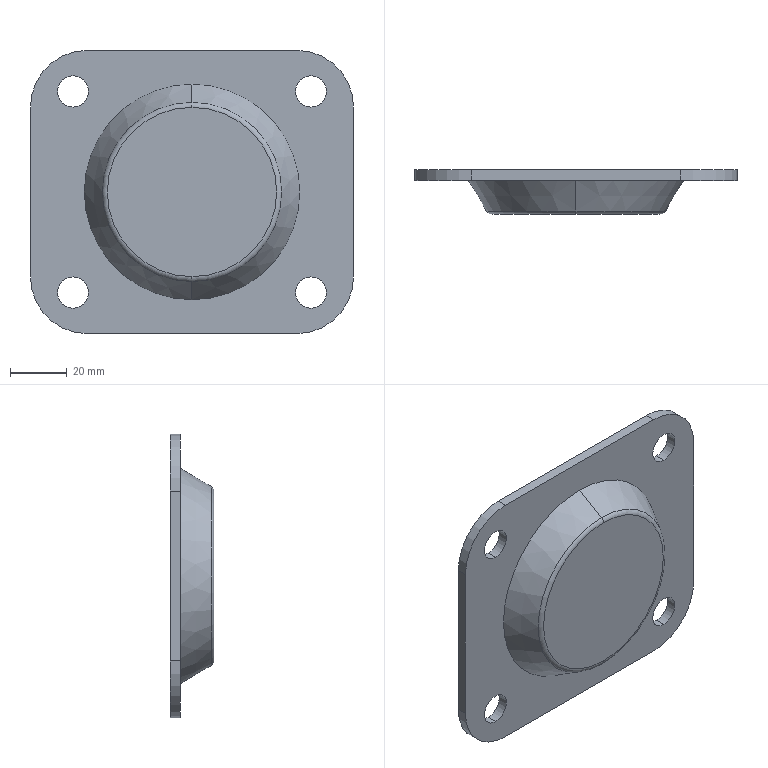Part | SolidWorks | features RefAxis 6, 3DProfileFeature 2, ICE 2, Extrusion 1, Revolution 1 | 1 solid | 26 faces | box 114 x 15.475 x 100 mm | volume 79826 mm3 | cylinder 14 | plane 8 | torus 2 | cone 2 | commonest cylinder face diameters 11 x8 40 x4 63.333 x2
STEP:
#1=CARTESIAN_POINT('',(-42.,-3.6,30.));
#2=VERTEX_POINT('',#1);
#3=CARTESIAN_POINT('',(-42.,-3.6,41.));
#4=VERTEX_POINT('',#3);
#5=CARTESIAN_POINT('',(-42.,-3.6,35.5));
#6=DIRECTION('',(0.,1.,0.));
#7=DIRECTION('',(0.,0.,1.));
#8=AXIS2_PLACEMENT_3D('',#5,#6,#7);
#9=CIRCLE('',#8,5.5);
#10=EDGE_CURVE('',#2,#4,#9,.T.);
#11=ORIENTED_EDGE('',*,*,#10,.F.);
#12=CARTESIAN_POINT('',(-42.,0.,30.));
#13=VERTEX_POINT('',#12);
#14=CARTESIAN_POINT('',(-42.,-15.475,30.));
#15=DIRECTION('',(0.,1.,0.));
#16=VECTOR('',#15,1000.);
#17=LINE('',#14,#16);
#18=EDGE_CURVE('',#2,#13,#17,.T.);
#19=ORIENTED_EDGE('',*,*,#18,.T.);
#20=CARTESIAN_POINT('',(-42.,0.,41.));
#21=VERTEX_POINT('',#20);
#22=CARTESIAN_POINT('',(-42.,0.,35.5));
#23=DIRECTION('',(0.,1.,0.));
#24=DIRECTION('',(0.,0.,-1.));
#25=AXIS2_PLACEMENT_3D('',#22,#23,#24);
#26=CIRCLE('',#25,5.5);
#27=EDGE_CURVE('',#13,#21,#26,.T.);
#28=ORIENTED_EDGE('',*,*,#27,.T.);
#29=CARTESIAN_POINT('',(-42.,-15.475,41.));
#30=DIRECTION('',(0.,1.,0.));
#31=VECTOR('',#30,1000.);
#32=LINE('',#29,#31);
#33=EDGE_CURVE('',#4,#21,#32,.T.);
#34=ORIENTED_EDGE('',*,*,#33,.F.);
#35=EDGE_LOOP('',(#11,#19,#28,#34));
#36=FACE_OUTER_BOUND('',#35,.T.);
#37=CARTESIAN_POINT('',(-42.,-15.475,35.5));
#38=DIRECTION('',(0.,1.,0.));
#39=DIRECTION('',(0.,0.,1.));
#40=AXIS2_PLACEMENT_3D('',#37,#38,#39);
#41=CYLINDRICAL_SURFACE('',#40,5.5);
#42=ADVANCED_FACE('',(#36),#41,.F.);
#43=CARTESIAN_POINT('',(42.,-3.6,30.));
#44=VERTEX_POINT('',#43);
#45=CARTESIAN_POINT('',(42.,-3.6,41.));
#46=VERTEX_POINT('',#45);
#47=CARTESIAN_POINT('',(42.,-3.6,35.5));
#48=DIRECTION('',(0.,1.,0.));
#49=DIRECTION('',(0.,0.,1.));
#50=AXIS2_PLACEMENT_3D('',#47,#48,#49);
#51=CIRCLE('',#50,5.5);
#52=EDGE_CURVE('',#44,#46,#51,.T.);
#53=ORIENTED_EDGE('',*,*,#52,.F.);
#54=CARTESIAN_POINT('',(42.,0.,30.));
#55=VERTEX_POINT('',#54);
#56=CARTESIAN_POINT('',(42.,-15.475,30.));
#57=DIRECTION('',(0.,1.,0.));
#58=VECTOR('',#57,1000.);
#59=LINE('',#56,#58);
#60=EDGE_CURVE('',#44,#55,#59,.T.);
#61=ORIENTED_EDGE('',*,*,#60,.T.);
#62=CARTESIAN_POINT('',(42.,0.,41.));
#63=VERTEX_POINT('',#62);
#64=CARTESIAN_POINT('',(42.,0.,35.5));
#65=DIRECTION('',(0.,1.,0.));
#66=DIRECTION('',(0.,0.,-1.));
#67=AXIS2_PLACEMENT_3D('',#64,#65,#66);
#68=CIRCLE('',#67,5.5);
#69=EDGE_CURVE('',#55,#63,#68,.T.);
#70=ORIENTED_EDGE('',*,*,#69,.T.);
#71=CARTESIAN_POINT('',(42.,-15.475,41.));
#72=DIRECTION('',(0.,1.,0.));
#73=VECTOR('',#72,1000.);
#74=LINE('',#71,#73);
#75=EDGE_CURVE('',#46,#63,#74,.T.);
#76=ORIENTED_EDGE('',*,*,#75,.F.);
#77=EDGE_LOOP('',(#53,#61,#70,#76));
#78=FACE_OUTER_BOUND('',#77,.T.);
#79=CARTESIAN_POINT('',(42.,-15.475,35.5));
#80=DIRECTION('',(0.,1.,0.));
#81=DIRECTION('',(0.,0.,1.));
#82=AXIS2_PLACEMENT_3D('',#79,#80,#81);
#83=CYLINDRICAL_SURFACE('',#82,5.5);
#84=ADVANCED_FACE('',(#78),#83,.F.);
#85=CARTESIAN_POINT('',(42.,-3.6,-41.));
#86=VERTEX_POINT('',#85);
#87=CARTESIAN_POINT('',(42.,-3.6,-30.));
#88=VERTEX_POINT('',#87);
#89=CARTESIAN_POINT('',(42.,-3.6,-35.5));
#90=DIRECTION('',(0.,1.,0.));
#91=DIRECTION('',(0.,0.,1.));
#92=AXIS2_PLACEMENT_3D('',#89,#90,#91);
#93=CIRCLE('',#92,5.5);
#94=EDGE_CURVE('',#86,#88,#93,.T.);
#95=ORIENTED_EDGE('',*,*,#94,.F.);
#96=CARTESIAN_POINT('',(42.,0.,-41.));
#97=VERTEX_POINT('',#96);
#98=CARTESIAN_POINT('',(42.,-15.475,-41.));
#99=DIRECTION('',(0.,1.,0.));
#100=VECTOR('',#99,1000.);
#101=LINE('',#98,#100);
#102=EDGE_CURVE('',#86,#97,#101,.T.);
#103=ORIENTED_EDGE('',*,*,#102,.T.);
#104=CARTESIAN_POINT('',(42.,0.,-30.));
#105=VERTEX_POINT('',#104);
#106=CARTESIAN_POINT('',(42.,0.,-35.5));
#107=DIRECTION('',(0.,1.,0.));
#108=DIRECTION('',(0.,0.,1.));
#109=AXIS2_PLACEMENT_3D('',#106,#107,#108);
#110=CIRCLE('',#109,5.5);
#111=EDGE_CURVE('',#97,#105,#110,.T.);
#112=ORIENTED_EDGE('',*,*,#111,.T.);
#113=CARTESIAN_POINT('',(42.,-15.475,-30.));
#114=DIRECTION('',(0.,1.,0.));
#115=VECTOR('',#114,1000.);
#116=LINE('',#113,#115);
#117=EDGE_CURVE('',#88,#105,#116,.T.);
#118=ORIENTED_EDGE('',*,*,#117,.F.);
#119=EDGE_LOOP('',(#95,#103,#112,#118));
#120=FACE_OUTER_BOUND('',#119,.T.);
#121=CARTESIAN_POINT('',(42.,-15.475,-35.5));
#122=DIRECTION('',(0.,1.,0.));
#123=DIRECTION('',(0.,0.,1.));
#124=AXIS2_PLACEMENT_3D('',#121,#122,#123);
#125=CYLINDRICAL_SURFACE('',#124,5.5);
#126=ADVANCED_FACE('',(#120),#125,.F.);
#127=CARTESIAN_POINT('',(-42.,-3.6,-41.));
#128=VERTEX_POINT('',#127);
#129=CARTESIAN_POINT('',(-42.,-3.6,-30.));
#130=VERTEX_POINT('',#129);
#131=CARTESIAN_POINT('',(-42.,-3.6,-35.5));
#132=DIRECTION('',(0.,1.,0.));
#133=DIRECTION('',(0.,0.,1.));
#134=AXIS2_PLACEMENT_3D('',#131,#132,#133);
#135=CIRCLE('',#134,5.5);
#136=EDGE_CURVE('',#128,#130,#135,.T.);
#137=ORIENTED_EDGE('',*,*,#136,.F.);
#138=CARTESIAN_POINT('',(-42.,0.,-41.));
#139=VERTEX_POINT('',#138);
#140=CARTESIAN_POINT('',(-42.,-15.475,-41.));
#141=DIRECTION('',(0.,1.,0.));
#142=VECTOR('',#141,1000.);
#143=LINE('',#140,#142);
#144=EDGE_CURVE('',#128,#139,#143,.T.);
#145=ORIENTED_EDGE('',*,*,#144,.T.);
#146=CARTESIAN_POINT('',(-42.,0.,-30.));
#147=VERTEX_POINT('',#146);
#148=CARTESIAN_POINT('',(-42.,0.,-35.5));
#149=DIRECTION('',(0.,1.,0.));
#150=DIRECTION('',(0.,0.,1.));
#151=AXIS2_PLACEMENT_3D('',#148,#149,#150);
#152=CIRCLE('',#151,5.5);
#153=EDGE_CURVE('',#139,#147,#152,.T.);
#154=ORIENTED_EDGE('',*,*,#153,.T.);
#155=CARTESIAN_POINT('',(-42.,-15.475,-30.));
#156=DIRECTION('',(0.,1.,0.));
#157=VECTOR('',#156,1000.);
#158=LINE('',#155,#157);
#159=EDGE_CURVE('',#130,#147,#158,.T.);
#160=ORIENTED_EDGE('',*,*,#159,.F.);
#161=EDGE_LOOP('',(#137,#145,#154,#160));
#162=FACE_OUTER_BOUND('',#161,.T.);
#163=CARTESIAN_POINT('',(-42.,-15.475,-35.5));
#164=DIRECTION('',(0.,1.,0.));
#165=DIRECTION('',(0.,0.,1.));
#166=AXIS2_PLACEMENT_3D('',#163,#164,#165);
#167=CYLINDRICAL_SURFACE('',#166,5.5);
#168=ADVANCED_FACE('',(#162),#167,.F.);
#169=CARTESIAN_POINT('',(0.,-15.475,29.876));
#170=VERTEX_POINT('',#169);
#171=CARTESIAN_POINT('',(0.,-15.475,-29.876));
#172=VERTEX_POINT('',#171);
#173=CARTESIAN_POINT('',(0.,-15.475,0.));
#174=DIRECTION('',(0.,1.,0.));
#175=DIRECTION('',(0.,0.,1.));
#176=AXIS2_PLACEMENT_3D('',#173,#174,#175);
#177=CIRCLE('',#176,29.876);
#178=EDGE_CURVE('',#170,#172,#177,.T.);
#179=ORIENTED_EDGE('',*,*,#178,.T.);
#180=CARTESIAN_POINT('',(0.,-14.488,-31.6));
#181=VERTEX_POINT('',#180);
#182=CARTESIAN_POINT('',(0.,-13.475,-29.876));
#183=DIRECTION('',(1.,0.,0.));
#184=DIRECTION('',(0.,0.,-1.));
#185=AXIS2_PLACEMENT_3D('',#182,#183,#184);
#186=CIRCLE('',#185,2.);
#187=EDGE_CURVE('',#172,#181,#186,.T.);
#188=ORIENTED_EDGE('',*,*,#187,.T.);
#189=CARTESIAN_POINT('',(0.,-14.488,31.6));
#190=VERTEX_POINT('',#189);
#191=CARTESIAN_POINT('',(0.,-14.488,0.));
#192=DIRECTION('',(0.,1.,0.));
#193=DIRECTION('',(0.,0.,1.));
#194=AXIS2_PLACEMENT_3D('',#191,#192,#193);
#195=CIRCLE('',#194,31.6);
#196=EDGE_CURVE('',#190,#181,#195,.T.);
#197=ORIENTED_EDGE('',*,*,#196,.F.);
#198=CARTESIAN_POINT('',(0.,-13.475,29.876));
#199=DIRECTION('',(-1.,0.,0.));
#200=DIRECTION('',(0.,0.,1.));
#201=AXIS2_PLACEMENT_3D('',#198,#199,#200);
#202=CIRCLE('',#201,2.);
#203=EDGE_CURVE('',#170,#190,#202,.T.);
#204=ORIENTED_EDGE('',*,*,#203,.F.);
#205=EDGE_LOOP('',(#179,#188,#197,#204));
#206=FACE_OUTER_BOUND('',#205,.T.);
#207=CARTESIAN_POINT('',(0.,-13.475,0.));
#208=DIRECTION('',(0.,1.,0.));
#209=DIRECTION('',(0.,0.,1.));
#210=AXIS2_PLACEMENT_3D('',#207,#208,#209);
#211=TOROIDAL_SURFACE('',#210,29.876,2.);
#212=ADVANCED_FACE('',(#206),#211,.T.);
#213=ORIENTED_EDGE('',*,*,#196,.T.);
#214=CARTESIAN_POINT('',(0.,-3.6,-38.));
#215=VERTEX_POINT('',#214);
#216=CARTESIAN_POINT('',(0.,-14.488,-31.6));
#217=DIRECTION('',(0.,0.8621,-0.5067));
#218=VECTOR('',#217,1000.);
#219=LINE('',#216,#218);
#220=EDGE_CURVE('',#181,#215,#219,.T.);
#221=ORIENTED_EDGE('',*,*,#220,.T.);
#222=CARTESIAN_POINT('',(0.,-3.6,38.));
#223=VERTEX_POINT('',#222);
#224=CARTESIAN_POINT('',(0.,-3.6,0.));
#225=DIRECTION('',(0.,-1.,0.));
#226=DIRECTION('',(0.,0.,1.));
#227=AXIS2_PLACEMENT_3D('',#224,#225,#226);
#228=CIRCLE('',#227,38.);
#229=EDGE_CURVE('',#215,#223,#228,.T.);
#230=ORIENTED_EDGE('',*,*,#229,.T.);
#231=CARTESIAN_POINT('',(0.,-14.488,31.6));
#232=DIRECTION('',(0.,0.8621,0.5067));
#233=VECTOR('',#232,1000.);
#234=LINE('',#231,#233);
#235=EDGE_CURVE('',#190,#223,#234,.T.);
#236=ORIENTED_EDGE('',*,*,#235,.F.);
#237=EDGE_LOOP('',(#213,#221,#230,#236));
#238=FACE_OUTER_BOUND('',#237,.T.);
#239=CARTESIAN_POINT('',(0.,-14.488,0.));
#240=DIRECTION('',(0.,1.,0.));
#241=DIRECTION('',(0.,0.,1.));
#242=AXIS2_PLACEMENT_3D('',#239,#240,#241);
#243=CONICAL_SURFACE('',#242,31.6,0.5314);
#244=ADVANCED_FACE('',(#238),#243,.T.);
#245=CARTESIAN_POINT('',(0.,-1.,-31.667));
#246=VERTEX_POINT('',#245);
#247=CARTESIAN_POINT('',(0.,-1.,31.667));
#248=VERTEX_POINT('',#247);
#249=CARTESIAN_POINT('',(0.,-1.,0.));
#250=DIRECTION('',(0.,1.,0.));
#251=DIRECTION('',(0.,0.,1.));
#252=AXIS2_PLACEMENT_3D('',#249,#250,#251);
#253=CIRCLE('',#252,31.667);
#254=EDGE_CURVE('',#246,#248,#253,.T.);
#255=ORIENTED_EDGE('',*,*,#254,.F.);
#256=CARTESIAN_POINT('',(0.,0.,-31.667));
#257=VERTEX_POINT('',#256);
#258=CARTESIAN_POINT('',(0.,-1.,-31.667));
#259=DIRECTION('',(0.,1.,0.));
#260=VECTOR('',#259,1000.);
#261=LINE('',#258,#260);
#262=EDGE_CURVE('',#246,#257,#261,.T.);
#263=ORIENTED_EDGE('',*,*,#262,.T.);
#264=CARTESIAN_POINT('',(0.,0.,31.667));
#265=VERTEX_POINT('',#264);
#266=CARTESIAN_POINT('',(0.,0.,0.));
#267=DIRECTION('',(0.,1.,0.));
#268=DIRECTION('',(0.,0.,1.));
#269=AXIS2_PLACEMENT_3D('',#266,#267,#268);
#270=CIRCLE('',#269,31.667);
#271=EDGE_CURVE('',#257,#265,#270,.T.);
#272=ORIENTED_EDGE('',*,*,#271,.T.);
#273=CARTESIAN_POINT('',(0.,-1.,31.667));
#274=DIRECTION('',(0.,1.,0.));
#275=VECTOR('',#274,1000.);
#276=LINE('',#273,#275);
#277=EDGE_CURVE('',#248,#265,#276,.T.);
#278=ORIENTED_EDGE('',*,*,#277,.F.);
#279=EDGE_LOOP('',(#255,#263,#272,#278));
#280=FACE_OUTER_BOUND('',#279,.T.);
#281=CARTESIAN_POINT('',(0.,-1.,0.));
#282=DIRECTION('',(0.,1.,0.));
#283=DIRECTION('',(0.,0.,1.));
#284=AXIS2_PLACEMENT_3D('',#281,#282,#283);
#285=CYLINDRICAL_SURFACE('',#284,31.667);
#286=ADVANCED_FACE('',(#280),#285,.F.);
#287=CARTESIAN_POINT('',(-42.,-3.6,35.5));
#288=DIRECTION('',(0.,1.,0.));
#289=DIRECTION('',(0.,0.,1.));
#290=AXIS2_PLACEMENT_3D('',#287,#288,#289);
#291=CIRCLE('',#290,5.5);
#292=EDGE_CURVE('',#4,#2,#291,.T.);
#293=ORIENTED_EDGE('',*,*,#292,.T.);
#294=ORIENTED_EDGE('',*,*,#10,.T.);
#295=EDGE_LOOP('',(#293,#294));
#296=FACE_BOUND('',#295,.T.);
#297=CARTESIAN_POINT('',(42.,-3.6,35.5));
#298=DIRECTION('',(0.,1.,0.));
#299=DIRECTION('',(0.,0.,1.));
#300=AXIS2_PLACEMENT_3D('',#297,#298,#299);
#301=CIRCLE('',#300,5.5);
#302=EDGE_CURVE('',#46,#44,#301,.T.);
#303=ORIENTED_EDGE('',*,*,#302,.T.);
#304=ORIENTED_EDGE('',*,*,#52,.T.);
#305=EDGE_LOOP('',(#303,#304));
#306=FACE_BOUND('',#305,.T.);
#307=CARTESIAN_POINT('',(42.,-3.6,-35.5));
#308=DIRECTION('',(0.,1.,0.));
#309=DIRECTION('',(0.,0.,1.));
#310=AXIS2_PLACEMENT_3D('',#307,#308,#309);
#311=CIRCLE('',#310,5.5);
#312=EDGE_CURVE('',#88,#86,#311,.T.);
#313=ORIENTED_EDGE('',*,*,#312,.T.);
#314=ORIENTED_EDGE('',*,*,#94,.T.);
#315=EDGE_LOOP('',(#313,#314));
#316=FACE_BOUND('',#315,.T.);
#317=CARTESIAN_POINT('',(-42.,-3.6,-35.5));
#318=DIRECTION('',(0.,1.,0.));
#319=DIRECTION('',(0.,0.,1.));
#320=AXIS2_PLACEMENT_3D('',#317,#318,#319);
#321=CIRCLE('',#320,5.5);
#322=EDGE_CURVE('',#130,#128,#321,.T.);
#323=ORIENTED_EDGE('',*,*,#322,.T.);
#324=ORIENTED_EDGE('',*,*,#136,.T.);
#325=EDGE_LOOP('',(#323,#324));
#326=FACE_BOUND('',#325,.T.);
#327=CARTESIAN_POINT('',(-57.,-3.6,30.));
#328=VERTEX_POINT('',#327);
#329=CARTESIAN_POINT('',(-37.,-3.6,50.));
#330=VERTEX_POINT('',#329);
#331=CARTESIAN_POINT('',(-37.,-3.6,30.));
#332=DIRECTION('',(0.,1.,0.));
#333=DIRECTION('',(0.,0.,1.));
#334=AXIS2_PLACEMENT_3D('',#331,#332,#333);
#335=CIRCLE('',#334,20.);
#336=EDGE_CURVE('',#328,#330,#335,.T.);
#337=ORIENTED_EDGE('',*,*,#336,.F.);
#338=CARTESIAN_POINT('',(-57.,-3.6,-30.));
#339=VERTEX_POINT('',#338);
#340=CARTESIAN_POINT('',(-57.,-3.6,-30.));
#341=DIRECTION('',(0.,0.,1.));
#342=VECTOR('',#341,1000.);
#343=LINE('',#340,#342);
#344=EDGE_CURVE('',#339,#328,#343,.T.);
#345=ORIENTED_EDGE('',*,*,#344,.F.);
#346=CARTESIAN_POINT('',(-37.,-3.6,-50.));
#347=VERTEX_POINT('',#346);
#348=CARTESIAN_POINT('',(-37.,-3.6,-30.));
#349=DIRECTION('',(0.,1.,0.));
#350=DIRECTION('',(0.,0.,1.));
#351=AXIS2_PLACEMENT_3D('',#348,#349,#350);
#352=CIRCLE('',#351,20.);
#353=EDGE_CURVE('',#347,#339,#352,.T.);
#354=ORIENTED_EDGE('',*,*,#353,.F.);
#355=CARTESIAN_POINT('',(37.,-3.6,-50.));
#356=VERTEX_POINT('',#355);
#357=CARTESIAN_POINT('',(-37.,-3.6,-50.));
#358=DIRECTION('',(-1.,0.,0.));
#359=VECTOR('',#358,1000.);
#360=LINE('',#357,#359);
#361=EDGE_CURVE('',#356,#347,#360,.T.);
#362=ORIENTED_EDGE('',*,*,#361,.F.);
#363=CARTESIAN_POINT('',(57.,-3.6,-30.));
#364=VERTEX_POINT('',#363);
#365=CARTESIAN_POINT('',(37.,-3.6,-30.));
#366=DIRECTION('',(0.,1.,0.));
#367=DIRECTION('',(0.,0.,-1.));
#368=AXIS2_PLACEMENT_3D('',#365,#366,#367);
#369=CIRCLE('',#368,20.);
#370=EDGE_CURVE('',#364,#356,#369,.T.);
#371=ORIENTED_EDGE('',*,*,#370,.F.);
#372=CARTESIAN_POINT('',(57.,-3.6,30.));
#373=VERTEX_POINT('',#372);
#374=CARTESIAN_POINT('',(57.,-3.6,-30.));
#375=DIRECTION('',(0.,0.,-1.));
#376=VECTOR('',#375,1000.);
#377=LINE('',#374,#376);
#378=EDGE_CURVE('',#373,#364,#377,.T.);
#379=ORIENTED_EDGE('',*,*,#378,.F.);
#380=CARTESIAN_POINT('',(37.,-3.6,50.));
#381=VERTEX_POINT('',#380);
#382=CARTESIAN_POINT('',(37.,-3.6,30.));
#383=DIRECTION('',(0.,1.,0.));
#384=DIRECTION('',(0.,0.,1.));
#385=AXIS2_PLACEMENT_3D('',#382,#383,#384);
#386=CIRCLE('',#385,20.);
#387=EDGE_CURVE('',#381,#373,#386,.T.);
#388=ORIENTED_EDGE('',*,*,#387,.F.);
#389=CARTESIAN_POINT('',(-37.,-3.6,50.));
#390=DIRECTION('',(1.,0.,0.));
#391=VECTOR('',#390,1000.);
#392=LINE('',#389,#391);
#393=EDGE_CURVE('',#330,#381,#392,.T.);
#394=ORIENTED_EDGE('',*,*,#393,.F.);
#395=EDGE_LOOP('',(#337,#345,#354,#362,#371,#379,#388,#394));
#396=FACE_OUTER_BOUND('',#395,.T.);
#397=CARTESIAN_POINT('',(0.,-3.6,0.));
#398=DIRECTION('',(0.,-1.,0.));
#399=DIRECTION('',(0.,0.,1.));
#400=AXIS2_PLACEMENT_3D('',#397,#398,#399);
#401=CIRCLE('',#400,38.);
#402=EDGE_CURVE('',#223,#215,#401,.T.);
#403=ORIENTED_EDGE('',*,*,#402,.F.);
#404=ORIENTED_EDGE('',*,*,#229,.F.);
#405=EDGE_LOOP('',(#403,#404));
#406=FACE_BOUND('',#405,.T.);
#407=CARTESIAN_POINT('',(-37.,-3.6,30.));
#408=DIRECTION('',(0.,1.,0.));
#409=DIRECTION('',(0.,0.,1.));
#410=AXIS2_PLACEMENT_3D('',#407,#408,#409);
#411=PLANE('',#410);
#412=ADVANCED_FACE('',(#296,#306,#316,#326,#396,#406),#411,.F.);
#413=CARTESIAN_POINT('',(-57.,0.,30.));
#414=VERTEX_POINT('',#413);
#415=CARTESIAN_POINT('',(-37.,0.,50.));
#416=VERTEX_POINT('',#415);
#417=CARTESIAN_POINT('',(-37.,0.,30.));
#418=DIRECTION('',(0.,1.,0.));
#419=DIRECTION('',(0.,0.,1.));
#420=AXIS2_PLACEMENT_3D('',#417,#418,#419);
#421=CIRCLE('',#420,20.);
#422=EDGE_CURVE('',#414,#416,#421,.T.);
#423=ORIENTED_EDGE('',*,*,#422,.F.);
#424=CARTESIAN_POINT('',(-57.,-3.6,30.));
#425=DIRECTION('',(0.,1.,0.));
#426=VECTOR('',#425,1000.);
#427=LINE('',#424,#426);
#428=EDGE_CURVE('',#328,#414,#427,.T.);
#429=ORIENTED_EDGE('',*,*,#428,.F.);
#430=ORIENTED_EDGE('',*,*,#336,.T.);
#431=CARTESIAN_POINT('',(-37.,-3.6,50.));
#432=DIRECTION('',(0.,1.,0.));
#433=VECTOR('',#432,1000.);
#434=LINE('',#431,#433);
#435=EDGE_CURVE('',#330,#416,#434,.T.);
#436=ORIENTED_EDGE('',*,*,#435,.T.);
#437=EDGE_LOOP('',(#423,#429,#430,#436));
#438=FACE_OUTER_BOUND('',#437,.T.);
#439=CARTESIAN_POINT('',(-37.,-3.6,30.));
#440=DIRECTION('',(0.,1.,0.));
#441=DIRECTION('',(0.,0.,1.));
#442=AXIS2_PLACEMENT_3D('',#439,#440,#441);
#443=CYLINDRICAL_SURFACE('',#442,20.);
#444=ADVANCED_FACE('',(#438),#443,.T.);
#445=CARTESIAN_POINT('',(-57.,0.,-30.));
#446=VERTEX_POINT('',#445);
#447=CARTESIAN_POINT('',(-57.,0.,-30.));
#448=DIRECTION('',(0.,0.,1.));
#449=VECTOR('',#448,1000.);
#450=LINE('',#447,#449);
#451=EDGE_CURVE('',#446,#414,#450,.T.);
#452=ORIENTED_EDGE('',*,*,#451,.F.);
#453=CARTESIAN_POINT('',(-57.,-3.6,-30.));
#454=DIRECTION('',(0.,1.,0.));
#455=VECTOR('',#454,1000.);
#456=LINE('',#453,#455);
#457=EDGE_CURVE('',#339,#446,#456,.T.);
#458=ORIENTED_EDGE('',*,*,#457,.F.);
#459=ORIENTED_EDGE('',*,*,#344,.T.);
#460=ORIENTED_EDGE('',*,*,#428,.T.);
#461=EDGE_LOOP('',(#452,#458,#459,#460));
#462=FACE_OUTER_BOUND('',#461,.T.);
#463=CARTESIAN_POINT('',(-57.,-3.6,-30.));
#464=DIRECTION('',(-1.,0.,0.));
#465=DIRECTION('',(0.,0.,1.));
#466=AXIS2_PLACEMENT_3D('',#463,#464,#465);
#467=PLANE('',#466);
#468=ADVANCED_FACE('',(#462),#467,.T.);
#469=CARTESIAN_POINT('',(-37.,0.,-50.));
#470=VERTEX_POINT('',#469);
#471=CARTESIAN_POINT('',(-37.,0.,-30.));
#472=DIRECTION('',(0.,1.,0.));
#473=DIRECTION('',(0.,0.,1.));
#474=AXIS2_PLACEMENT_3D('',#471,#472,#473);
#475=CIRCLE('',#474,20.);
#476=EDGE_CURVE('',#470,#446,#475,.T.);
#477=ORIENTED_EDGE('',*,*,#476,.F.);
#478=CARTESIAN_POINT('',(-37.,-3.6,-50.));
#479=DIRECTION('',(0.,1.,0.));
#480=VECTOR('',#479,1000.);
#481=LINE('',#478,#480);
#482=EDGE_CURVE('',#347,#470,#481,.T.);
#483=ORIENTED_EDGE('',*,*,#482,.F.);
#484=ORIENTED_EDGE('',*,*,#353,.T.);
#485=ORIENTED_EDGE('',*,*,#457,.T.);
#486=EDGE_LOOP('',(#477,#483,#484,#485));
#487=FACE_OUTER_BOUND('',#486,.T.);
#488=CARTESIAN_POINT('',(-37.,-3.6,-30.));
#489=DIRECTION('',(0.,1.,0.));
#490=DIRECTION('',(0.,0.,1.));
#491=AXIS2_PLACEMENT_3D('',#488,#489,#490);
#492=CYLINDRICAL_SURFACE('',#491,20.);
#493=ADVANCED_FACE('',(#487),#492,.T.);
#494=CARTESIAN_POINT('',(37.,0.,-50.));
#495=VERTEX_POINT('',#494);
#496=CARTESIAN_POINT('',(-37.,0.,-50.));
#497=DIRECTION('',(-1.,0.,0.));
#498=VECTOR('',#497,1000.);
#499=LINE('',#496,#498);
#500=EDGE_CURVE('',#495,#470,#499,.T.);
#501=ORIENTED_EDGE('',*,*,#500,.F.);
#502=CARTESIAN_POINT('',(37.,-3.6,-50.));
#503=DIRECTION('',(0.,1.,0.));
#504=VECTOR('',#503,1000.);
#505=LINE('',#502,#504);
#506=EDGE_CURVE('',#356,#495,#505,.T.);
#507=ORIENTED_EDGE('',*,*,#506,.F.);
#508=ORIENTED_EDGE('',*,*,#361,.T.);
#509=ORIENTED_EDGE('',*,*,#482,.T.);
#510=EDGE_LOOP('',(#501,#507,#508,#509));
#511=FACE_OUTER_BOUND('',#510,.T.);
#512=CARTESIAN_POINT('',(-37.,-3.6,-50.));
#513=DIRECTION('',(0.,0.,-1.));
#514=DIRECTION('',(-1.,0.,0.));
#515=AXIS2_PLACEMENT_3D('',#512,#513,#514);
#516=PLANE('',#515);
#517=ADVANCED_FACE('',(#511),#516,.T.);
#518=CARTESIAN_POINT('',(57.,0.,-30.));
#519=VERTEX_POINT('',#518);
#520=CARTESIAN_POINT('',(37.,0.,-30.));
#521=DIRECTION('',(0.,1.,0.));
#522=DIRECTION('',(0.,0.,-1.));
#523=AXIS2_PLACEMENT_3D('',#520,#521,#522);
#524=CIRCLE('',#523,20.);
#525=EDGE_CURVE('',#519,#495,#524,.T.);
#526=ORIENTED_EDGE('',*,*,#525,.F.);
#527=CARTESIAN_POINT('',(57.,-3.6,-30.));
#528=DIRECTION('',(0.,1.,0.));
#529=VECTOR('',#528,1000.);
#530=LINE('',#527,#529);
#531=EDGE_CURVE('',#364,#519,#530,.T.);
#532=ORIENTED_EDGE('',*,*,#531,.F.);
#533=ORIENTED_EDGE('',*,*,#370,.T.);
#534=ORIENTED_EDGE('',*,*,#506,.T.);
#535=EDGE_LOOP('',(#526,#532,#533,#534));
#536=FACE_OUTER_BOUND('',#535,.T.);
#537=CARTESIAN_POINT('',(37.,-3.6,-30.));
#538=DIRECTION('',(0.,1.,0.));
#539=DIRECTION('',(0.,0.,1.));
#540=AXIS2_PLACEMENT_3D('',#537,#538,#539);
#541=CYLINDRICAL_SURFACE('',#540,20.);
#542=ADVANCED_FACE('',(#536),#541,.T.);
#543=CARTESIAN_POINT('',(57.,0.,30.));
#544=VERTEX_POINT('',#543);
#545=CARTESIAN_POINT('',(57.,0.,-30.));
#546=DIRECTION('',(0.,0.,-1.));
#547=VECTOR('',#546,1000.);
#548=LINE('',#545,#547);
#549=EDGE_CURVE('',#544,#519,#548,.T.);
#550=ORIENTED_EDGE('',*,*,#549,.F.);
#551=CARTESIAN_POINT('',(57.,-3.6,30.));
#552=DIRECTION('',(0.,1.,0.));
#553=VECTOR('',#552,1000.);
#554=LINE('',#551,#553);
#555=EDGE_CURVE('',#373,#544,#554,.T.);
#556=ORIENTED_EDGE('',*,*,#555,.F.);
#557=ORIENTED_EDGE('',*,*,#378,.T.);
#558=ORIENTED_EDGE('',*,*,#531,.T.);
#559=EDGE_LOOP('',(#550,#556,#557,#558));
#560=FACE_OUTER_BOUND('',#559,.T.);
#561=CARTESIAN_POINT('',(57.,-3.6,-30.));
#562=DIRECTION('',(1.,0.,0.));
#563=DIRECTION('',(0.,0.,-1.));
#564=AXIS2_PLACEMENT_3D('',#561,#562,#563);
#565=PLANE('',#564);
#566=ADVANCED_FACE('',(#560),#565,.T.);
#567=CARTESIAN_POINT('',(37.,0.,50.));
#568=VERTEX_POINT('',#567);
#569=CARTESIAN_POINT('',(37.,0.,30.));
#570=DIRECTION('',(0.,1.,0.));
#571=DIRECTION('',(0.,0.,1.));
#572=AXIS2_PLACEMENT_3D('',#569,#570,#571);
#573=CIRCLE('',#572,20.);
#574=EDGE_CURVE('',#568,#544,#573,.T.);
#575=ORIENTED_EDGE('',*,*,#574,.F.);
#576=CARTESIAN_POINT('',(37.,-3.6,50.));
#577=DIRECTION('',(0.,1.,0.));
#578=VECTOR('',#577,1000.);
#579=LINE('',#576,#578);
#580=EDGE_CURVE('',#381,#568,#579,.T.);
#581=ORIENTED_EDGE('',*,*,#580,.F.);
#582=ORIENTED_EDGE('',*,*,#387,.T.);
#583=ORIENTED_EDGE('',*,*,#555,.T.);
#584=EDGE_LOOP('',(#575,#581,#582,#583));
#585=FACE_OUTER_BOUND('',#584,.T.);
#586=CARTESIAN_POINT('',(37.,-3.6,30.));
#587=DIRECTION('',(0.,1.,0.));
#588=DIRECTION('',(0.,0.,1.));
#589=AXIS2_PLACEMENT_3D('',#586,#587,#588);
#590=CYLINDRICAL_SURFACE('',#589,20.);
#591=ADVANCED_FACE('',(#585),#590,.T.);
#592=CARTESIAN_POINT('',(-37.,0.,50.));
#593=DIRECTION('',(1.,0.,0.));
#594=VECTOR('',#593,1000.);
#595=LINE('',#592,#594);
#596=EDGE_CURVE('',#416,#568,#595,.T.);
#597=ORIENTED_EDGE('',*,*,#596,.F.);
#598=ORIENTED_EDGE('',*,*,#435,.F.);
#599=ORIENTED_EDGE('',*,*,#393,.T.);
#600=ORIENTED_EDGE('',*,*,#580,.T.);
#601=EDGE_LOOP('',(#597,#598,#599,#600));
#602=FACE_OUTER_BOUND('',#601,.T.);
#603=CARTESIAN_POINT('',(-37.,-3.6,50.));
#604=DIRECTION('',(0.,0.,1.));
#605=DIRECTION('',(1.,0.,0.));
#606=AXIS2_PLACEMENT_3D('',#603,#604,#605);
#607=PLANE('',#606);
#608=ADVANCED_FACE('',(#602),#607,.T.);
#609=CARTESIAN_POINT('',(-42.,0.,35.5));
#610=DIRECTION('',(0.,1.,0.));
#611=DIRECTION('',(0.,0.,-1.));
#612=AXIS2_PLACEMENT_3D('',#609,#610,#611);
#613=CIRCLE('',#612,5.5);
#614=EDGE_CURVE('',#21,#13,#613,.T.);
#615=ORIENTED_EDGE('',*,*,#614,.F.);
#616=ORIENTED_EDGE('',*,*,#27,.F.);
#617=EDGE_LOOP('',(#615,#616));
#618=FACE_BOUND('',#617,.T.);
#619=CARTESIAN_POINT('',(42.,0.,35.5));
#620=DIRECTION('',(0.,1.,0.));
#621=DIRECTION('',(0.,0.,-1.));
#622=AXIS2_PLACEMENT_3D('',#619,#620,#621);
#623=CIRCLE('',#622,5.5);
#624=EDGE_CURVE('',#63,#55,#623,.T.);
#625=ORIENTED_EDGE('',*,*,#624,.F.);
#626=ORIENTED_EDGE('',*,*,#69,.F.);
#627=EDGE_LOOP('',(#625,#626));
#628=FACE_BOUND('',#627,.T.);
#629=CARTESIAN_POINT('',(42.,0.,-35.5));
#630=DIRECTION('',(0.,1.,0.));
#631=DIRECTION('',(0.,0.,1.));
#632=AXIS2_PLACEMENT_3D('',#629,#630,#631);
#633=CIRCLE('',#632,5.5);
#634=EDGE_CURVE('',#105,#97,#633,.T.);
#635=ORIENTED_EDGE('',*,*,#634,.F.);
#636=ORIENTED_EDGE('',*,*,#111,.F.);
#637=EDGE_LOOP('',(#635,#636));
#638=FACE_BOUND('',#637,.T.);
#639=CARTESIAN_POINT('',(-42.,0.,-35.5));
#640=DIRECTION('',(0.,1.,0.));
#641=DIRECTION('',(0.,0.,1.));
#642=AXIS2_PLACEMENT_3D('',#639,#640,#641);
#643=CIRCLE('',#642,5.5);
#644=EDGE_CURVE('',#147,#139,#643,.T.);
#645=ORIENTED_EDGE('',*,*,#644,.F.);
#646=ORIENTED_EDGE('',*,*,#153,.F.);
#647=EDGE_LOOP('',(#645,#646));
#648=FACE_BOUND('',#647,.T.);
#649=CARTESIAN_POINT('',(0.,0.,0.));
#650=DIRECTION('',(0.,1.,0.));
#651=DIRECTION('',(0.,0.,1.));
#652=AXIS2_PLACEMENT_3D('',#649,#650,#651);
#653=CIRCLE('',#652,31.667);
#654=EDGE_CURVE('',#265,#257,#653,.T.);
#655=ORIENTED_EDGE('',*,*,#654,.F.);
#656=ORIENTED_EDGE('',*,*,#271,.F.);
#657=EDGE_LOOP('',(#655,#656));
#658=FACE_BOUND('',#657,.T.);
#659=ORIENTED_EDGE('',*,*,#422,.T.);
#660=ORIENTED_EDGE('',*,*,#596,.T.);
#661=ORIENTED_EDGE('',*,*,#574,.T.);
#662=ORIENTED_EDGE('',*,*,#549,.T.);
#663=ORIENTED_EDGE('',*,*,#525,.T.);
#664=ORIENTED_EDGE('',*,*,#500,.T.);
#665=ORIENTED_EDGE('',*,*,#476,.T.);
#666=ORIENTED_EDGE('',*,*,#451,.T.);
#667=EDGE_LOOP('',(#659,#660,#661,#662,#663,#664,#665,#666));
#668=FACE_OUTER_BOUND('',#667,.T.);
#669=CARTESIAN_POINT('',(-37.,0.,30.));
#670=DIRECTION('',(0.,1.,0.));
#671=DIRECTION('',(0.,0.,1.));
#672=AXIS2_PLACEMENT_3D('',#669,#670,#671);
#673=PLANE('',#672);
#674=ADVANCED_FACE('',(#618,#628,#638,#648,#658,#668),#673,.T.);
#675=ORIENTED_EDGE('',*,*,#262,.F.);
#676=CARTESIAN_POINT('',(0.,-1.,0.));
#677=DIRECTION('',(0.,1.,0.));
#678=DIRECTION('',(0.,0.,1.));
#679=AXIS2_PLACEMENT_3D('',#676,#677,#678);
#680=CIRCLE('',#679,31.667);
#681=EDGE_CURVE('',#248,#246,#680,.T.);
#682=ORIENTED_EDGE('',*,*,#681,.F.);
#683=ORIENTED_EDGE('',*,*,#277,.T.);
#684=ORIENTED_EDGE('',*,*,#654,.T.);
#685=EDGE_LOOP('',(#675,#682,#683,#684));
#686=FACE_OUTER_BOUND('',#685,.T.);
#687=CARTESIAN_POINT('',(0.,-1.,0.));
#688=DIRECTION('',(0.,1.,0.));
#689=DIRECTION('',(0.,0.,1.));
#690=AXIS2_PLACEMENT_3D('',#687,#688,#689);
#691=CYLINDRICAL_SURFACE('',#690,31.667);
#692=ADVANCED_FACE('',(#686),#691,.F.);
#693=ORIENTED_EDGE('',*,*,#681,.T.);
#694=ORIENTED_EDGE('',*,*,#254,.T.);
#695=EDGE_LOOP('',(#693,#694));
#696=FACE_OUTER_BOUND('',#695,.T.);
#697=CARTESIAN_POINT('',(0.,-1.,0.));
#698=DIRECTION('',(0.,1.,0.));
#699=DIRECTION('',(0.,0.,1.));
#700=AXIS2_PLACEMENT_3D('',#697,#698,#699);
#701=PLANE('',#700);
#702=ADVANCED_FACE('',(#696),#701,.T.);
#703=ORIENTED_EDGE('',*,*,#220,.F.);
#704=CARTESIAN_POINT('',(0.,-14.488,0.));
#705=DIRECTION('',(0.,1.,0.));
#706=DIRECTION('',(0.,0.,1.));
#707=AXIS2_PLACEMENT_3D('',#704,#705,#706);
#708=CIRCLE('',#707,31.6);
#709=EDGE_CURVE('',#181,#190,#708,.T.);
#710=ORIENTED_EDGE('',*,*,#709,.T.);
#711=ORIENTED_EDGE('',*,*,#235,.T.);
#712=ORIENTED_EDGE('',*,*,#402,.T.);
#713=EDGE_LOOP('',(#703,#710,#711,#712));
#714=FACE_OUTER_BOUND('',#713,.T.);
#715=CARTESIAN_POINT('',(0.,-14.488,0.));
#716=DIRECTION('',(0.,1.,0.));
#717=DIRECTION('',(0.,0.,1.));
#718=AXIS2_PLACEMENT_3D('',#715,#716,#717);
#719=CONICAL_SURFACE('',#718,31.6,0.5314);
#720=ADVANCED_FACE('',(#714),#719,.T.);
#721=ORIENTED_EDGE('',*,*,#187,.F.);
#722=CARTESIAN_POINT('',(0.,-15.475,0.));
#723=DIRECTION('',(0.,1.,0.));
#724=DIRECTION('',(0.,0.,1.));
#725=AXIS2_PLACEMENT_3D('',#722,#723,#724);
#726=CIRCLE('',#725,29.876);
#727=EDGE_CURVE('',#172,#170,#726,.T.);
#728=ORIENTED_EDGE('',*,*,#727,.T.);
#729=ORIENTED_EDGE('',*,*,#203,.T.);
#730=ORIENTED_EDGE('',*,*,#709,.F.);
#731=EDGE_LOOP('',(#721,#728,#729,#730));
#732=FACE_OUTER_BOUND('',#731,.T.);
#733=CARTESIAN_POINT('',(0.,-13.475,0.));
#734=DIRECTION('',(0.,1.,0.));
#735=DIRECTION('',(0.,0.,1.));
#736=AXIS2_PLACEMENT_3D('',#733,#734,#735);
#737=TOROIDAL_SURFACE('',#736,29.876,2.);
#738=ADVANCED_FACE('',(#732),#737,.T.);
#739=ORIENTED_EDGE('',*,*,#178,.F.);
#740=ORIENTED_EDGE('',*,*,#727,.F.);
#741=EDGE_LOOP('',(#739,#740));
#742=FACE_OUTER_BOUND('',#741,.T.);
#743=CARTESIAN_POINT('',(29.876,-15.475,0.));
#744=DIRECTION('',(0.,1.,0.));
#745=DIRECTION('',(0.,0.,1.));
#746=AXIS2_PLACEMENT_3D('',#743,#744,#745);
#747=PLANE('',#746);
#748=ADVANCED_FACE('',(#742),#747,.F.);
#749=ORIENTED_EDGE('',*,*,#144,.F.);
#750=ORIENTED_EDGE('',*,*,#322,.F.);
#751=ORIENTED_EDGE('',*,*,#159,.T.);
#752=ORIENTED_EDGE('',*,*,#644,.T.);
#753=EDGE_LOOP('',(#749,#750,#751,#752));
#754=FACE_OUTER_BOUND('',#753,.T.);
#755=CARTESIAN_POINT('',(-42.,-15.475,-35.5));
#756=DIRECTION('',(0.,1.,0.));
#757=DIRECTION('',(0.,0.,1.));
#758=AXIS2_PLACEMENT_3D('',#755,#756,#757);
#759=CYLINDRICAL_SURFACE('',#758,5.5);
#760=ADVANCED_FACE('',(#754),#759,.F.);
#761=ORIENTED_EDGE('',*,*,#102,.F.);
#762=ORIENTED_EDGE('',*,*,#312,.F.);
#763=ORIENTED_EDGE('',*,*,#117,.T.);
#764=ORIENTED_EDGE('',*,*,#634,.T.);
#765=EDGE_LOOP('',(#761,#762,#763,#764));
#766=FACE_OUTER_BOUND('',#765,.T.);
#767=CARTESIAN_POINT('',(42.,-15.475,-35.5));
#768=DIRECTION('',(0.,1.,0.));
#769=DIRECTION('',(0.,0.,1.));
#770=AXIS2_PLACEMENT_3D('',#767,#768,#769);
#771=CYLINDRICAL_SURFACE('',#770,5.5);
#772=ADVANCED_FACE('',(#766),#771,.F.);
#773=ORIENTED_EDGE('',*,*,#60,.F.);
#774=ORIENTED_EDGE('',*,*,#302,.F.);
#775=ORIENTED_EDGE('',*,*,#75,.T.);
#776=ORIENTED_EDGE('',*,*,#624,.T.);
#777=EDGE_LOOP('',(#773,#774,#775,#776));
#778=FACE_OUTER_BOUND('',#777,.T.);
#779=CARTESIAN_POINT('',(42.,-15.475,35.5));
#780=DIRECTION('',(0.,1.,0.));
#781=DIRECTION('',(0.,0.,1.));
#782=AXIS2_PLACEMENT_3D('',#779,#780,#781);
#783=CYLINDRICAL_SURFACE('',#782,5.5);
#784=ADVANCED_FACE('',(#778),#783,.F.);
#785=ORIENTED_EDGE('',*,*,#18,.F.);
#786=ORIENTED_EDGE('',*,*,#292,.F.);
#787=ORIENTED_EDGE('',*,*,#33,.T.);
#788=ORIENTED_EDGE('',*,*,#614,.T.);
#789=EDGE_LOOP('',(#785,#786,#787,#788));
#790=FACE_OUTER_BOUND('',#789,.T.);
#791=CARTESIAN_POINT('',(-42.,-15.475,35.5));
#792=DIRECTION('',(0.,1.,0.));
#793=DIRECTION('',(0.,0.,1.));
#794=AXIS2_PLACEMENT_3D('',#791,#792,#793);
#795=CYLINDRICAL_SURFACE('',#794,5.5);
#796=ADVANCED_FACE('',(#790),#795,.F.);
#797=CLOSED_SHELL('',(#42,#84,#126,#168,#212,#244,#286,#412,#444,#468,#493,#517,#542,#566,#591,#608,#674,#692,#702,#720,#738,#748,#760,#772,#784,#796));
#798=MANIFOLD_SOLID_BREP('',#797);
#799=CARTESIAN_POINT('',(0.,0.,0.));
#800=DIRECTION('',(0.,0.,1.));
#801=DIRECTION('',(1.,0.,0.));
#802=AXIS2_PLACEMENT_3D('',#799,#800,#801);
#803=(LENGTH_UNIT()NAMED_UNIT(*)SI_UNIT(.MILLI.,.METRE.));
#804=UNCERTAINTY_MEASURE_WITH_UNIT(LENGTH_MEASURE(0.00001),#803,'','');
#805=(NAMED_UNIT(*)PLANE_ANGLE_UNIT()SI_UNIT($,.RADIAN.));
#806=(NAMED_UNIT(*)SI_UNIT($,.STERADIAN.)SOLID_ANGLE_UNIT());
#807=(GEOMETRIC_REPRESENTATION_CONTEXT(3)GLOBAL_UNCERTAINTY_ASSIGNED_CONTEXT((#804))GLOBAL_UNIT_ASSIGNED_CONTEXT((#803,#805,#806))REPRESENTATION_CONTEXT('',''));
#808=ADVANCED_BREP_SHAPE_REPRESENTATION('',(#798,#802),#807);